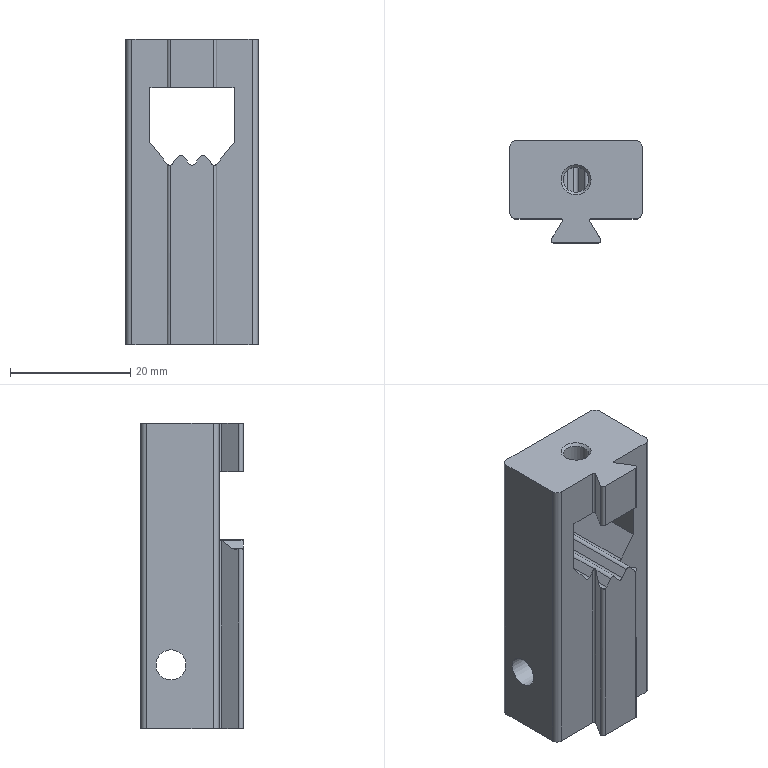Part | STEP file | 200 mesh_id2162 | 1 solid | 46 faces | box 22 x 17 x 50.8 mm | volume 12810 mm3 | plane 24 | cylinder 21 | cone 1 | commonest cylinder face diameters 1.04 x5 0.6 x4 1 x4 2 x4 1.2 x2 4.2 x1